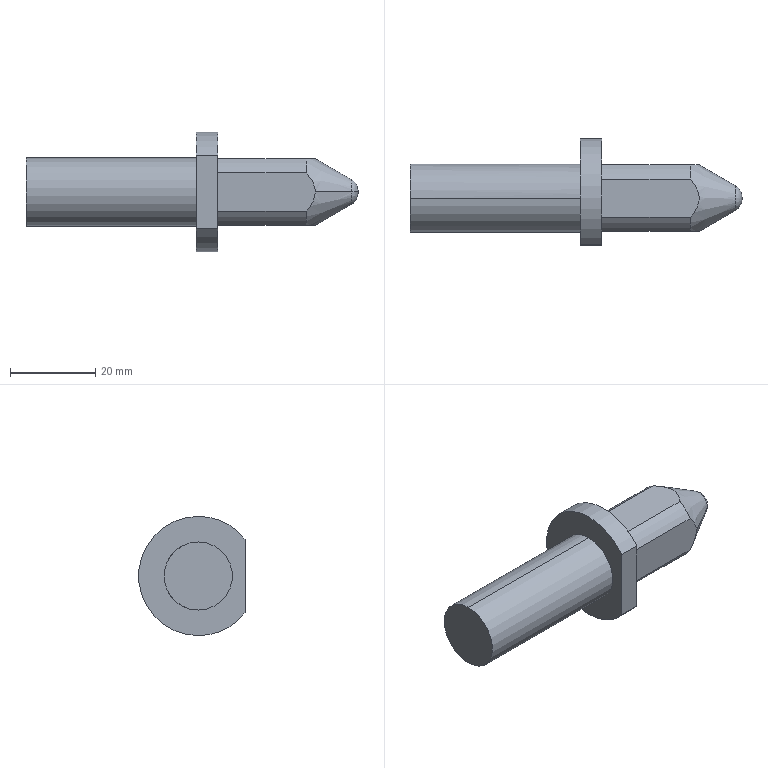Part | STEP file | Positioning_id1810_x_t | 1 solid | 20 faces | box 78 x 25 x 28 mm | volume 16926 mm3 | plane 9 | cylinder 7 | spline 2 | cone 2 | commonest cylinder face diameters 18 x4 16 x2 28 x1